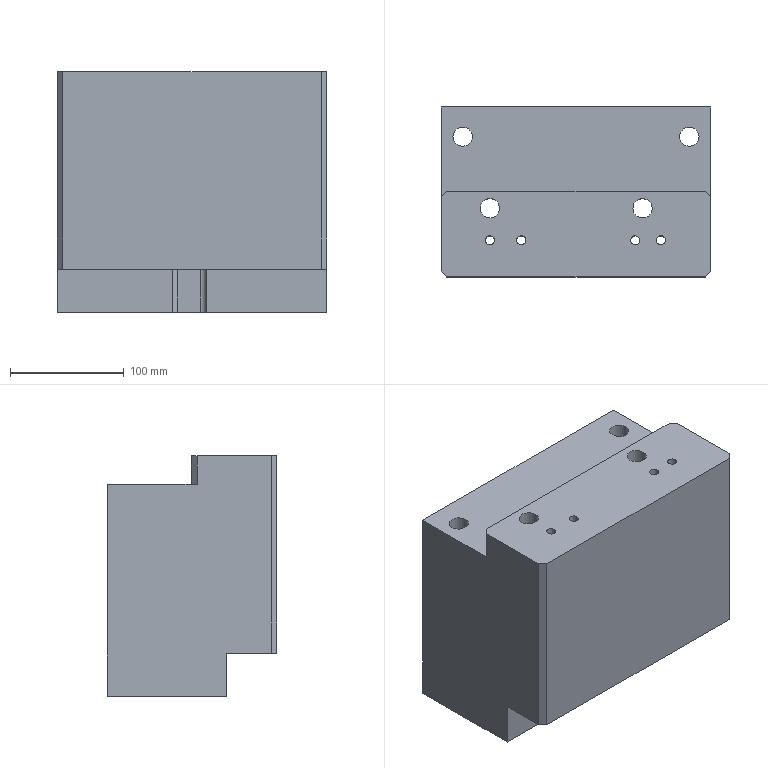Part | NX | features solid 2 | 1 solid | 56 faces | box 237 x 149 x 211 mm | volume 6174628 mm3 | plane 24 | cylinder 19 | cone 10 | spline 3 | commonest cylinder face diameters 8.5 x4 17 x4 26 x4 6 x2 10 x2 10.506 x2